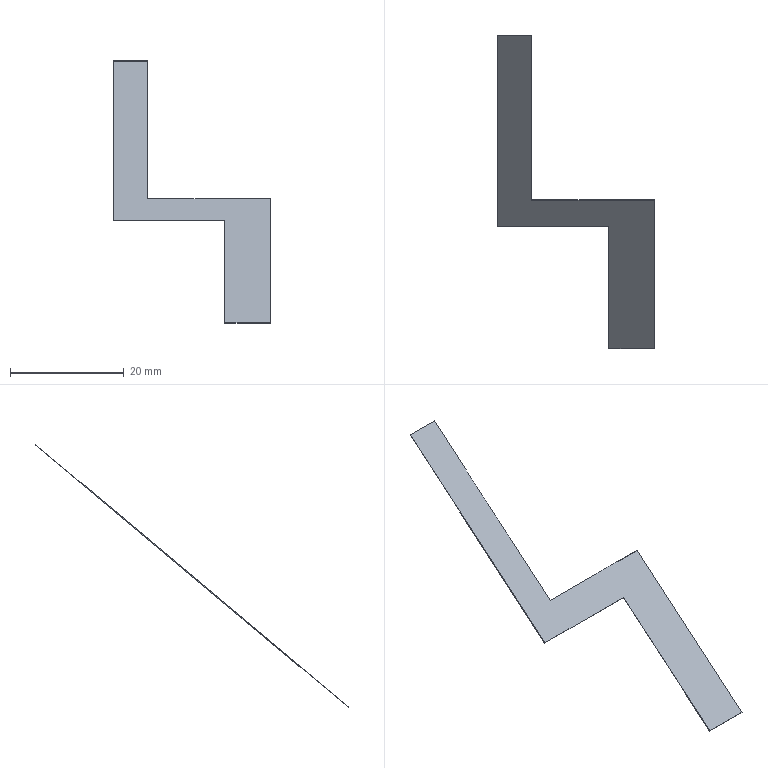Part | SolidWorks | features BaseBody 1 | 1 solid | 10 faces | box 27.548 x 54.936 x 46.114 mm | volume 46.14 mm3 | plane 10
STEP:
#1=CARTESIAN_POINT('',(-790.999,660.402,371.569));
#2=VERTEX_POINT('',#1);
#3=CARTESIAN_POINT('',(-790.999,693.841,399.627));
#4=VERTEX_POINT('',#3);
#5=CARTESIAN_POINT('',(-790.999,660.402,371.569));
#6=DIRECTION('',(-0.000001286,0.766,0.6428));
#7=VECTOR('',#6,1000.);
#8=LINE('',#5,#7);
#9=EDGE_CURVE('',#2,#4,#8,.T.);
#10=ORIENTED_EDGE('',*,*,#9,.F.);
#11=CARTESIAN_POINT('',(-790.999,660.353,371.626));
#12=VERTEX_POINT('',#11);
#13=CARTESIAN_POINT('',(-790.999,660.353,371.626));
#14=DIRECTION('',(-0.000000993,0.6428,-0.766));
#15=VECTOR('',#14,1000.);
#16=LINE('',#13,#15);
#17=EDGE_CURVE('',#12,#2,#16,.T.);
#18=ORIENTED_EDGE('',*,*,#17,.F.);
#19=CARTESIAN_POINT('',(-790.999,693.792,399.685));
#20=VERTEX_POINT('',#19);
#21=CARTESIAN_POINT('',(-790.999,693.792,399.685));
#22=DIRECTION('',(0.000001286,-0.766,-0.6428));
#23=VECTOR('',#22,1000.);
#24=LINE('',#21,#23);
#25=EDGE_CURVE('',#20,#12,#24,.T.);
#26=ORIENTED_EDGE('',*,*,#25,.F.);
#27=CARTESIAN_POINT('',(-790.999,693.841,399.627));
#28=DIRECTION('',(0.000000993,-0.6428,0.766));
#29=VECTOR('',#28,1000.);
#30=LINE('',#27,#29);
#31=EDGE_CURVE('',#4,#20,#30,.T.);
#32=ORIENTED_EDGE('',*,*,#31,.F.);
#33=EDGE_LOOP('',(#10,#18,#26,#32));
#34=FACE_OUTER_BOUND('',#33,.T.);
#35=CARTESIAN_POINT('',(-790.999,660.402,371.569));
#36=DIRECTION('',(1.,0.000001623,0.000000066));
#37=DIRECTION('',(-0.000001286,0.766,0.6428));
#38=AXIS2_PLACEMENT_3D('',#35,#36,#37);
#39=PLANE('',#38);
#40=ADVANCED_FACE('',(#34),#39,.F.);
#41=CARTESIAN_POINT('',(-784.999,693.841,399.627));
#42=VERTEX_POINT('',#41);
#43=CARTESIAN_POINT('',(-790.999,693.841,399.627));
#44=DIRECTION('',(1.,0.000001623,0.000000066));
#45=VECTOR('',#44,1000.);
#46=LINE('',#43,#45);
#47=EDGE_CURVE('',#4,#42,#46,.T.);
#48=ORIENTED_EDGE('',*,*,#47,.F.);
#49=ORIENTED_EDGE('',*,*,#31,.T.);
#50=CARTESIAN_POINT('',(-784.999,693.792,399.685));
#51=VERTEX_POINT('',#50);
#52=CARTESIAN_POINT('',(-790.999,693.792,399.685));
#53=DIRECTION('',(1.,0.000001623,0.000000066));
#54=VECTOR('',#53,1000.);
#55=LINE('',#52,#54);
#56=EDGE_CURVE('',#20,#51,#55,.T.);
#57=ORIENTED_EDGE('',*,*,#56,.T.);
#58=CARTESIAN_POINT('',(-784.999,693.841,399.627));
#59=DIRECTION('',(0.000000993,-0.6428,0.766));
#60=VECTOR('',#59,1000.);
#61=LINE('',#58,#60);
#62=EDGE_CURVE('',#42,#51,#61,.T.);
#63=ORIENTED_EDGE('',*,*,#62,.F.);
#64=EDGE_LOOP('',(#48,#49,#57,#63));
#65=FACE_OUTER_BOUND('',#64,.T.);
#66=CARTESIAN_POINT('',(-790.999,693.841,399.627));
#67=DIRECTION('',(0.000001286,-0.766,-0.6428));
#68=DIRECTION('',(0.000000993,-0.6428,0.766));
#69=AXIS2_PLACEMENT_3D('',#66,#67,#68);
#70=PLANE('',#69);
#71=ADVANCED_FACE('',(#65),#70,.F.);
#72=CARTESIAN_POINT('',(-784.999,664.998,375.425));
#73=VERTEX_POINT('',#72);
#74=CARTESIAN_POINT('',(-784.999,664.998,375.425));
#75=DIRECTION('',(-0.000001286,0.766,0.6428));
#76=VECTOR('',#75,1000.);
#77=LINE('',#74,#76);
#78=EDGE_CURVE('',#73,#42,#77,.T.);
#79=ORIENTED_EDGE('',*,*,#78,.T.);
#80=ORIENTED_EDGE('',*,*,#62,.T.);
#81=CARTESIAN_POINT('',(-784.999,664.95,375.483));
#82=VERTEX_POINT('',#81);
#83=CARTESIAN_POINT('',(-784.999,693.792,399.685));
#84=DIRECTION('',(0.000001286,-0.766,-0.6428));
#85=VECTOR('',#84,1000.);
#86=LINE('',#83,#85);
#87=EDGE_CURVE('',#51,#82,#86,.T.);
#88=ORIENTED_EDGE('',*,*,#87,.T.);
#89=CARTESIAN_POINT('',(-784.999,664.95,375.483));
#90=DIRECTION('',(-0.000000993,0.6428,-0.766));
#91=VECTOR('',#90,1000.);
#92=LINE('',#89,#91);
#93=EDGE_CURVE('',#82,#73,#92,.T.);
#94=ORIENTED_EDGE('',*,*,#93,.T.);
#95=EDGE_LOOP('',(#79,#80,#88,#94));
#96=FACE_OUTER_BOUND('',#95,.T.);
#97=CARTESIAN_POINT('',(-784.999,693.841,399.627));
#98=DIRECTION('',(-1.,-0.000001623,-0.000000066));
#99=DIRECTION('',(0.000001286,-0.766,-0.6428));
#100=AXIS2_PLACEMENT_3D('',#97,#98,#99);
#101=PLANE('',#100);
#102=ADVANCED_FACE('',(#96),#101,.F.);
#103=CARTESIAN_POINT('',(-763.451,664.998,375.425));
#104=VERTEX_POINT('',#103);
#105=CARTESIAN_POINT('',(-763.451,664.998,375.425));
#106=DIRECTION('',(-1.,-0.000001623,-0.000000066));
#107=VECTOR('',#106,1000.);
#108=LINE('',#105,#107);
#109=EDGE_CURVE('',#104,#73,#108,.T.);
#110=ORIENTED_EDGE('',*,*,#109,.T.);
#111=ORIENTED_EDGE('',*,*,#93,.F.);
#112=CARTESIAN_POINT('',(-763.451,664.95,375.483));
#113=VERTEX_POINT('',#112);
#114=CARTESIAN_POINT('',(-784.999,664.95,375.483));
#115=DIRECTION('',(1.,0.000001623,0.000000066));
#116=VECTOR('',#115,1000.);
#117=LINE('',#114,#116);
#118=EDGE_CURVE('',#82,#113,#117,.T.);
#119=ORIENTED_EDGE('',*,*,#118,.T.);
#120=CARTESIAN_POINT('',(-763.451,664.95,375.483));
#121=DIRECTION('',(-0.000000993,0.6428,-0.766));
#122=VECTOR('',#121,1000.);
#123=LINE('',#120,#122);
#124=EDGE_CURVE('',#113,#104,#123,.T.);
#125=ORIENTED_EDGE('',*,*,#124,.T.);
#126=EDGE_LOOP('',(#110,#111,#119,#125));
#127=FACE_OUTER_BOUND('',#126,.T.);
#128=CARTESIAN_POINT('',(-784.999,664.998,375.425));
#129=DIRECTION('',(0.000001286,-0.766,-0.6428));
#130=DIRECTION('',(1.,0.000001623,0.000000066));
#131=AXIS2_PLACEMENT_3D('',#128,#129,#130);
#132=PLANE('',#131);
#133=ADVANCED_FACE('',(#127),#132,.F.);
#134=CARTESIAN_POINT('',(-763.451,638.952,353.571));
#135=VERTEX_POINT('',#134);
#136=CARTESIAN_POINT('',(-763.451,638.952,353.571));
#137=DIRECTION('',(-0.000001286,0.766,0.6428));
#138=VECTOR('',#137,1000.);
#139=LINE('',#136,#138);
#140=EDGE_CURVE('',#135,#104,#139,.T.);
#141=ORIENTED_EDGE('',*,*,#140,.T.);
#142=ORIENTED_EDGE('',*,*,#124,.F.);
#143=CARTESIAN_POINT('',(-763.451,638.904,353.628));
#144=VERTEX_POINT('',#143);
#145=CARTESIAN_POINT('',(-763.451,664.95,375.483));
#146=DIRECTION('',(0.000001286,-0.766,-0.6428));
#147=VECTOR('',#146,1000.);
#148=LINE('',#145,#147);
#149=EDGE_CURVE('',#113,#144,#148,.T.);
#150=ORIENTED_EDGE('',*,*,#149,.T.);
#151=CARTESIAN_POINT('',(-763.451,638.904,353.628));
#152=DIRECTION('',(-0.000000993,0.6428,-0.766));
#153=VECTOR('',#152,1000.);
#154=LINE('',#151,#153);
#155=EDGE_CURVE('',#144,#135,#154,.T.);
#156=ORIENTED_EDGE('',*,*,#155,.T.);
#157=EDGE_LOOP('',(#141,#142,#150,#156));
#158=FACE_OUTER_BOUND('',#157,.T.);
#159=CARTESIAN_POINT('',(-763.451,664.998,375.425));
#160=DIRECTION('',(-1.,-0.000001623,-0.000000066));
#161=DIRECTION('',(0.000001286,-0.766,-0.6428));
#162=AXIS2_PLACEMENT_3D('',#159,#160,#161);
#163=PLANE('',#162);
#164=ADVANCED_FACE('',(#158),#163,.F.);
#165=CARTESIAN_POINT('',(-771.451,638.952,353.571));
#166=VERTEX_POINT('',#165);
#167=CARTESIAN_POINT('',(-771.451,638.952,353.571));
#168=DIRECTION('',(1.,0.000001623,0.000000066));
#169=VECTOR('',#168,1000.);
#170=LINE('',#167,#169);
#171=EDGE_CURVE('',#166,#135,#170,.T.);
#172=ORIENTED_EDGE('',*,*,#171,.T.);
#173=ORIENTED_EDGE('',*,*,#155,.F.);
#174=CARTESIAN_POINT('',(-771.451,638.904,353.628));
#175=VERTEX_POINT('',#174);
#176=CARTESIAN_POINT('',(-763.451,638.904,353.628));
#177=DIRECTION('',(-1.,-0.000001623,-0.000000066));
#178=VECTOR('',#177,1000.);
#179=LINE('',#176,#178);
#180=EDGE_CURVE('',#144,#175,#179,.T.);
#181=ORIENTED_EDGE('',*,*,#180,.T.);
#182=CARTESIAN_POINT('',(-771.451,638.904,353.628));
#183=DIRECTION('',(-0.000000993,0.6428,-0.766));
#184=VECTOR('',#183,1000.);
#185=LINE('',#182,#184);
#186=EDGE_CURVE('',#175,#166,#185,.T.);
#187=ORIENTED_EDGE('',*,*,#186,.T.);
#188=EDGE_LOOP('',(#172,#173,#181,#187));
#189=FACE_OUTER_BOUND('',#188,.T.);
#190=CARTESIAN_POINT('',(-763.451,638.952,353.571));
#191=DIRECTION('',(-0.000001286,0.766,0.6428));
#192=DIRECTION('',(-1.,-0.000001623,-0.000000066));
#193=AXIS2_PLACEMENT_3D('',#190,#191,#192);
#194=PLANE('',#193);
#195=ADVANCED_FACE('',(#189),#194,.F.);
#196=CARTESIAN_POINT('',(-771.451,660.402,371.569));
#197=VERTEX_POINT('',#196);
#198=CARTESIAN_POINT('',(-771.451,660.402,371.569));
#199=DIRECTION('',(0.000001286,-0.766,-0.6428));
#200=VECTOR('',#199,1000.);
#201=LINE('',#198,#200);
#202=EDGE_CURVE('',#197,#166,#201,.T.);
#203=ORIENTED_EDGE('',*,*,#202,.T.);
#204=ORIENTED_EDGE('',*,*,#186,.F.);
#205=CARTESIAN_POINT('',(-771.451,660.353,371.626));
#206=VERTEX_POINT('',#205);
#207=CARTESIAN_POINT('',(-771.451,638.904,353.628));
#208=DIRECTION('',(-0.000001286,0.766,0.6428));
#209=VECTOR('',#208,1000.);
#210=LINE('',#207,#209);
#211=EDGE_CURVE('',#175,#206,#210,.T.);
#212=ORIENTED_EDGE('',*,*,#211,.T.);
#213=CARTESIAN_POINT('',(-771.451,660.353,371.626));
#214=DIRECTION('',(-0.000000993,0.6428,-0.766));
#215=VECTOR('',#214,1000.);
#216=LINE('',#213,#215);
#217=EDGE_CURVE('',#206,#197,#216,.T.);
#218=ORIENTED_EDGE('',*,*,#217,.T.);
#219=EDGE_LOOP('',(#203,#204,#212,#218));
#220=FACE_OUTER_BOUND('',#219,.T.);
#221=CARTESIAN_POINT('',(-771.451,645.081,358.713));
#222=DIRECTION('',(1.,0.000001623,0.000000066));
#223=DIRECTION('',(-0.000001286,0.766,0.6428));
#224=AXIS2_PLACEMENT_3D('',#221,#222,#223);
#225=PLANE('',#224);
#226=ADVANCED_FACE('',(#220),#225,.F.);
#227=CARTESIAN_POINT('',(-790.999,660.402,371.569));
#228=DIRECTION('',(1.,0.000001623,0.000000066));
#229=VECTOR('',#228,1000.);
#230=LINE('',#227,#229);
#231=EDGE_CURVE('',#2,#197,#230,.T.);
#232=ORIENTED_EDGE('',*,*,#231,.T.);
#233=ORIENTED_EDGE('',*,*,#217,.F.);
#234=CARTESIAN_POINT('',(-771.451,660.353,371.626));
#235=DIRECTION('',(-1.,-0.000001623,-0.000000066));
#236=VECTOR('',#235,1000.);
#237=LINE('',#234,#236);
#238=EDGE_CURVE('',#206,#12,#237,.T.);
#239=ORIENTED_EDGE('',*,*,#238,.T.);
#240=ORIENTED_EDGE('',*,*,#17,.T.);
#241=EDGE_LOOP('',(#232,#233,#239,#240));
#242=FACE_OUTER_BOUND('',#241,.T.);
#243=CARTESIAN_POINT('',(-771.451,660.402,371.569));
#244=DIRECTION('',(-0.000001286,0.766,0.6428));
#245=DIRECTION('',(-0.000000993,0.6428,-0.766));
#246=AXIS2_PLACEMENT_3D('',#243,#244,#245);
#247=PLANE('',#246);
#248=ADVANCED_FACE('',(#242),#247,.F.);
#249=ORIENTED_EDGE('',*,*,#211,.F.);
#250=ORIENTED_EDGE('',*,*,#180,.F.);
#251=ORIENTED_EDGE('',*,*,#149,.F.);
#252=ORIENTED_EDGE('',*,*,#118,.F.);
#253=ORIENTED_EDGE('',*,*,#87,.F.);
#254=ORIENTED_EDGE('',*,*,#56,.F.);
#255=ORIENTED_EDGE('',*,*,#25,.T.);
#256=ORIENTED_EDGE('',*,*,#238,.F.);
#257=EDGE_LOOP('',(#249,#250,#251,#252,#253,#254,#255,#256));
#258=FACE_OUTER_BOUND('',#257,.T.);
#259=CARTESIAN_POINT('',(-733.13,689.217,395.846));
#260=DIRECTION('',(-0.000000993,0.6428,-0.766));
#261=DIRECTION('',(-1.,-0.000001623,-0.000000066));
#262=AXIS2_PLACEMENT_3D('',#259,#260,#261);
#263=PLANE('',#262);
#264=ADVANCED_FACE('',(#258),#263,.F.);
#265=ORIENTED_EDGE('',*,*,#78,.F.);
#266=ORIENTED_EDGE('',*,*,#109,.F.);
#267=ORIENTED_EDGE('',*,*,#140,.F.);
#268=ORIENTED_EDGE('',*,*,#171,.F.);
#269=ORIENTED_EDGE('',*,*,#202,.F.);
#270=ORIENTED_EDGE('',*,*,#231,.F.);
#271=ORIENTED_EDGE('',*,*,#9,.T.);
#272=ORIENTED_EDGE('',*,*,#47,.T.);
#273=EDGE_LOOP('',(#265,#266,#267,#268,#269,#270,#271,#272));
#274=FACE_OUTER_BOUND('',#273,.T.);
#275=CARTESIAN_POINT('',(-733.13,689.266,395.788));
#276=DIRECTION('',(-0.000000993,0.6428,-0.766));
#277=DIRECTION('',(-1.,-0.000001623,-0.000000066));
#278=AXIS2_PLACEMENT_3D('',#275,#276,#277);
#279=PLANE('',#278);
#280=ADVANCED_FACE('',(#274),#279,.T.);
#281=CLOSED_SHELL('',(#40,#71,#102,#133,#164,#195,#226,#248,#264,#280));
#282=MANIFOLD_SOLID_BREP('',#281);
#283=CARTESIAN_POINT('',(0.,0.,0.));
#284=DIRECTION('',(0.,0.,1.));
#285=DIRECTION('',(1.,0.,0.));
#286=AXIS2_PLACEMENT_3D('',#283,#284,#285);
#287=(LENGTH_UNIT()NAMED_UNIT(*)SI_UNIT(.MILLI.,.METRE.));
#288=UNCERTAINTY_MEASURE_WITH_UNIT(LENGTH_MEASURE(0.00001),#287,'','');
#289=(NAMED_UNIT(*)PLANE_ANGLE_UNIT()SI_UNIT($,.RADIAN.));
#290=(NAMED_UNIT(*)SI_UNIT($,.STERADIAN.)SOLID_ANGLE_UNIT());
#291=(GEOMETRIC_REPRESENTATION_CONTEXT(3)GLOBAL_UNCERTAINTY_ASSIGNED_CONTEXT((#288))GLOBAL_UNIT_ASSIGNED_CONTEXT((#287,#289,#290))REPRESENTATION_CONTEXT('',''));
#292=ADVANCED_BREP_SHAPE_REPRESENTATION('',(#282,#286),#291);